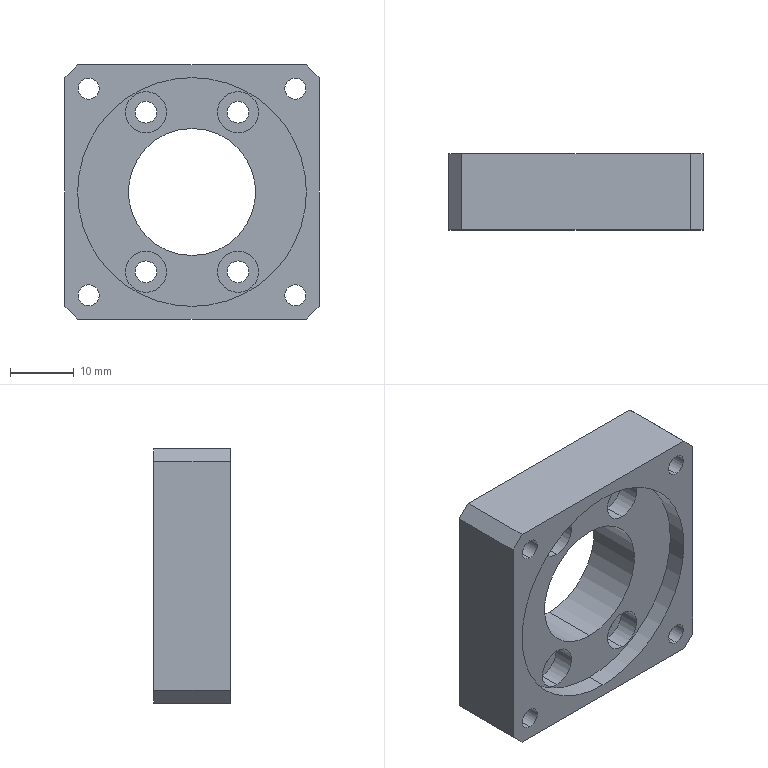Part | STEP file | 06-11 motor flange | 1 solid | 43 faces | box 40 x 12 x 40 mm | volume 12158 mm3 | cylinder 28 | plane 15 | commonest cylinder face diameters 3.3 x8 3.4 x8 6.5 x8 20 x2 36 x2
STEP:
#1=CARTESIAN_POINT('',(-16.263,12.,17.913));
#2=VERTEX_POINT('',#1);
#3=CARTESIAN_POINT('',(-16.263,12.,14.613));
#4=VERTEX_POINT('',#3);
#5=CARTESIAN_POINT('',(-16.263,12.,16.263));
#6=DIRECTION('',(0.,-1.,0.));
#7=DIRECTION('',(0.,0.,-1.));
#8=AXIS2_PLACEMENT_3D('',#5,#6,#7);
#9=CIRCLE('',#8,1.65);
#10=EDGE_CURVE('',#2,#4,#9,.T.);
#11=ORIENTED_EDGE('',*,*,#10,.F.);
#12=CARTESIAN_POINT('',(-16.263,0.,17.913));
#13=VERTEX_POINT('',#12);
#14=CARTESIAN_POINT('',(-16.263,0.,17.913));
#15=DIRECTION('',(0.,-1.,0.));
#16=VECTOR('',#15,1000.);
#17=LINE('',#14,#16);
#18=EDGE_CURVE('',#2,#13,#17,.T.);
#19=ORIENTED_EDGE('',*,*,#18,.T.);
#20=CARTESIAN_POINT('',(-16.263,0.,14.613));
#21=VERTEX_POINT('',#20);
#22=CARTESIAN_POINT('',(-16.263,0.,16.263));
#23=DIRECTION('',(0.,-1.,0.));
#24=DIRECTION('',(0.,0.,-1.));
#25=AXIS2_PLACEMENT_3D('',#22,#23,#24);
#26=CIRCLE('',#25,1.65);
#27=EDGE_CURVE('',#13,#21,#26,.T.);
#28=ORIENTED_EDGE('',*,*,#27,.T.);
#29=CARTESIAN_POINT('',(-16.263,0.,14.613));
#30=DIRECTION('',(0.,-1.,0.));
#31=VECTOR('',#30,1000.);
#32=LINE('',#29,#31);
#33=EDGE_CURVE('',#4,#21,#32,.T.);
#34=ORIENTED_EDGE('',*,*,#33,.F.);
#35=EDGE_LOOP('',(#11,#19,#28,#34));
#36=FACE_OUTER_BOUND('',#35,.T.);
#37=CARTESIAN_POINT('',(-16.263,0.,16.263));
#38=DIRECTION('',(0.,-1.,0.));
#39=DIRECTION('',(0.,0.,-1.));
#40=AXIS2_PLACEMENT_3D('',#37,#38,#39);
#41=CYLINDRICAL_SURFACE('',#40,1.65);
#42=ADVANCED_FACE('',(#36),#41,.F.);
#43=CARTESIAN_POINT('',(-16.263,12.,-14.613));
#44=VERTEX_POINT('',#43);
#45=CARTESIAN_POINT('',(-16.263,12.,-17.913));
#46=VERTEX_POINT('',#45);
#47=CARTESIAN_POINT('',(-16.263,12.,-16.263));
#48=DIRECTION('',(0.,-1.,0.));
#49=DIRECTION('',(0.,0.,-1.));
#50=AXIS2_PLACEMENT_3D('',#47,#48,#49);
#51=CIRCLE('',#50,1.65);
#52=EDGE_CURVE('',#44,#46,#51,.T.);
#53=ORIENTED_EDGE('',*,*,#52,.F.);
#54=CARTESIAN_POINT('',(-16.263,0.,-14.613));
#55=VERTEX_POINT('',#54);
#56=CARTESIAN_POINT('',(-16.263,0.,-14.613));
#57=DIRECTION('',(0.,-1.,0.));
#58=VECTOR('',#57,1000.);
#59=LINE('',#56,#58);
#60=EDGE_CURVE('',#44,#55,#59,.T.);
#61=ORIENTED_EDGE('',*,*,#60,.T.);
#62=CARTESIAN_POINT('',(-16.263,0.,-17.913));
#63=VERTEX_POINT('',#62);
#64=CARTESIAN_POINT('',(-16.263,0.,-16.263));
#65=DIRECTION('',(0.,-1.,0.));
#66=DIRECTION('',(0.,0.,-1.));
#67=AXIS2_PLACEMENT_3D('',#64,#65,#66);
#68=CIRCLE('',#67,1.65);
#69=EDGE_CURVE('',#55,#63,#68,.T.);
#70=ORIENTED_EDGE('',*,*,#69,.T.);
#71=CARTESIAN_POINT('',(-16.263,0.,-17.913));
#72=DIRECTION('',(0.,-1.,0.));
#73=VECTOR('',#72,1000.);
#74=LINE('',#71,#73);
#75=EDGE_CURVE('',#46,#63,#74,.T.);
#76=ORIENTED_EDGE('',*,*,#75,.F.);
#77=EDGE_LOOP('',(#53,#61,#70,#76));
#78=FACE_OUTER_BOUND('',#77,.T.);
#79=CARTESIAN_POINT('',(-16.263,0.,-16.263));
#80=DIRECTION('',(0.,-1.,0.));
#81=DIRECTION('',(0.,0.,-1.));
#82=AXIS2_PLACEMENT_3D('',#79,#80,#81);
#83=CYLINDRICAL_SURFACE('',#82,1.65);
#84=ADVANCED_FACE('',(#78),#83,.F.);
#85=CARTESIAN_POINT('',(16.263,12.,-14.613));
#86=VERTEX_POINT('',#85);
#87=CARTESIAN_POINT('',(16.263,12.,-17.913));
#88=VERTEX_POINT('',#87);
#89=CARTESIAN_POINT('',(16.263,12.,-16.263));
#90=DIRECTION('',(0.,-1.,0.));
#91=DIRECTION('',(0.,0.,-1.));
#92=AXIS2_PLACEMENT_3D('',#89,#90,#91);
#93=CIRCLE('',#92,1.65);
#94=EDGE_CURVE('',#86,#88,#93,.T.);
#95=ORIENTED_EDGE('',*,*,#94,.F.);
#96=CARTESIAN_POINT('',(16.263,0.,-14.613));
#97=VERTEX_POINT('',#96);
#98=CARTESIAN_POINT('',(16.263,0.,-14.613));
#99=DIRECTION('',(0.,-1.,0.));
#100=VECTOR('',#99,1000.);
#101=LINE('',#98,#100);
#102=EDGE_CURVE('',#86,#97,#101,.T.);
#103=ORIENTED_EDGE('',*,*,#102,.T.);
#104=CARTESIAN_POINT('',(16.263,0.,-17.913));
#105=VERTEX_POINT('',#104);
#106=CARTESIAN_POINT('',(16.263,0.,-16.263));
#107=DIRECTION('',(0.,-1.,0.));
#108=DIRECTION('',(0.,0.,-1.));
#109=AXIS2_PLACEMENT_3D('',#106,#107,#108);
#110=CIRCLE('',#109,1.65);
#111=EDGE_CURVE('',#97,#105,#110,.T.);
#112=ORIENTED_EDGE('',*,*,#111,.T.);
#113=CARTESIAN_POINT('',(16.263,0.,-17.913));
#114=DIRECTION('',(0.,-1.,0.));
#115=VECTOR('',#114,1000.);
#116=LINE('',#113,#115);
#117=EDGE_CURVE('',#88,#105,#116,.T.);
#118=ORIENTED_EDGE('',*,*,#117,.F.);
#119=EDGE_LOOP('',(#95,#103,#112,#118));
#120=FACE_OUTER_BOUND('',#119,.T.);
#121=CARTESIAN_POINT('',(16.263,0.,-16.263));
#122=DIRECTION('',(0.,-1.,0.));
#123=DIRECTION('',(0.,0.,-1.));
#124=AXIS2_PLACEMENT_3D('',#121,#122,#123);
#125=CYLINDRICAL_SURFACE('',#124,1.65);
#126=ADVANCED_FACE('',(#120),#125,.F.);
#127=CARTESIAN_POINT('',(16.263,12.,17.913));
#128=VERTEX_POINT('',#127);
#129=CARTESIAN_POINT('',(16.263,12.,14.613));
#130=VERTEX_POINT('',#129);
#131=CARTESIAN_POINT('',(16.263,12.,16.263));
#132=DIRECTION('',(0.,-1.,0.));
#133=DIRECTION('',(0.,0.,-1.));
#134=AXIS2_PLACEMENT_3D('',#131,#132,#133);
#135=CIRCLE('',#134,1.65);
#136=EDGE_CURVE('',#128,#130,#135,.T.);
#137=ORIENTED_EDGE('',*,*,#136,.F.);
#138=CARTESIAN_POINT('',(16.263,0.,17.913));
#139=VERTEX_POINT('',#138);
#140=CARTESIAN_POINT('',(16.263,0.,17.913));
#141=DIRECTION('',(0.,-1.,0.));
#142=VECTOR('',#141,1000.);
#143=LINE('',#140,#142);
#144=EDGE_CURVE('',#128,#139,#143,.T.);
#145=ORIENTED_EDGE('',*,*,#144,.T.);
#146=CARTESIAN_POINT('',(16.263,0.,14.613));
#147=VERTEX_POINT('',#146);
#148=CARTESIAN_POINT('',(16.263,0.,16.263));
#149=DIRECTION('',(0.,-1.,0.));
#150=DIRECTION('',(0.,0.,-1.));
#151=AXIS2_PLACEMENT_3D('',#148,#149,#150);
#152=CIRCLE('',#151,1.65);
#153=EDGE_CURVE('',#139,#147,#152,.T.);
#154=ORIENTED_EDGE('',*,*,#153,.T.);
#155=CARTESIAN_POINT('',(16.263,0.,14.613));
#156=DIRECTION('',(0.,-1.,0.));
#157=VECTOR('',#156,1000.);
#158=LINE('',#155,#157);
#159=EDGE_CURVE('',#130,#147,#158,.T.);
#160=ORIENTED_EDGE('',*,*,#159,.F.);
#161=EDGE_LOOP('',(#137,#145,#154,#160));
#162=FACE_OUTER_BOUND('',#161,.T.);
#163=CARTESIAN_POINT('',(16.263,0.,16.263));
#164=DIRECTION('',(0.,-1.,0.));
#165=DIRECTION('',(0.,0.,-1.));
#166=AXIS2_PLACEMENT_3D('',#163,#164,#165);
#167=CYLINDRICAL_SURFACE('',#166,1.65);
#168=ADVANCED_FACE('',(#162),#167,.F.);
#169=CARTESIAN_POINT('',(7.25,6.4,15.807));
#170=VERTEX_POINT('',#169);
#171=CARTESIAN_POINT('',(7.25,6.4,9.307));
#172=VERTEX_POINT('',#171);
#173=CARTESIAN_POINT('',(7.25,6.4,12.557));
#174=DIRECTION('',(0.,-1.,0.));
#175=DIRECTION('',(0.,0.,-1.));
#176=AXIS2_PLACEMENT_3D('',#173,#174,#175);
#177=CIRCLE('',#176,3.25);
#178=EDGE_CURVE('',#170,#172,#177,.T.);
#179=ORIENTED_EDGE('',*,*,#178,.F.);
#180=CARTESIAN_POINT('',(7.25,3.,15.807));
#181=VERTEX_POINT('',#180);
#182=CARTESIAN_POINT('',(7.25,3.,15.807));
#183=DIRECTION('',(0.,-1.,0.));
#184=VECTOR('',#183,1000.);
#185=LINE('',#182,#184);
#186=EDGE_CURVE('',#170,#181,#185,.T.);
#187=ORIENTED_EDGE('',*,*,#186,.T.);
#188=CARTESIAN_POINT('',(7.25,3.,9.307));
#189=VERTEX_POINT('',#188);
#190=CARTESIAN_POINT('',(7.25,3.,12.557));
#191=DIRECTION('',(0.,-1.,0.));
#192=DIRECTION('',(0.,0.,-1.));
#193=AXIS2_PLACEMENT_3D('',#190,#191,#192);
#194=CIRCLE('',#193,3.25);
#195=EDGE_CURVE('',#181,#189,#194,.T.);
#196=ORIENTED_EDGE('',*,*,#195,.T.);
#197=CARTESIAN_POINT('',(7.25,3.,9.307));
#198=DIRECTION('',(0.,-1.,0.));
#199=VECTOR('',#198,1000.);
#200=LINE('',#197,#199);
#201=EDGE_CURVE('',#172,#189,#200,.T.);
#202=ORIENTED_EDGE('',*,*,#201,.F.);
#203=EDGE_LOOP('',(#179,#187,#196,#202));
#204=FACE_OUTER_BOUND('',#203,.T.);
#205=CARTESIAN_POINT('',(7.25,3.,12.557));
#206=DIRECTION('',(0.,-1.,0.));
#207=DIRECTION('',(0.,0.,-1.));
#208=AXIS2_PLACEMENT_3D('',#205,#206,#207);
#209=CYLINDRICAL_SURFACE('',#208,3.25);
#210=ADVANCED_FACE('',(#204),#209,.F.);
#211=CARTESIAN_POINT('',(7.25,12.,14.257));
#212=VERTEX_POINT('',#211);
#213=CARTESIAN_POINT('',(7.25,12.,10.857));
#214=VERTEX_POINT('',#213);
#215=CARTESIAN_POINT('',(7.25,12.,12.557));
#216=DIRECTION('',(0.,-1.,0.));
#217=DIRECTION('',(0.,0.,-1.));
#218=AXIS2_PLACEMENT_3D('',#215,#216,#217);
#219=CIRCLE('',#218,1.7);
#220=EDGE_CURVE('',#212,#214,#219,.T.);
#221=ORIENTED_EDGE('',*,*,#220,.F.);
#222=CARTESIAN_POINT('',(7.25,6.4,14.257));
#223=VERTEX_POINT('',#222);
#224=CARTESIAN_POINT('',(7.25,3.,14.257));
#225=DIRECTION('',(0.,-1.,0.));
#226=VECTOR('',#225,1000.);
#227=LINE('',#224,#226);
#228=EDGE_CURVE('',#212,#223,#227,.T.);
#229=ORIENTED_EDGE('',*,*,#228,.T.);
#230=CARTESIAN_POINT('',(7.25,6.4,10.857));
#231=VERTEX_POINT('',#230);
#232=CARTESIAN_POINT('',(7.25,6.4,12.557));
#233=DIRECTION('',(0.,-1.,0.));
#234=DIRECTION('',(0.,0.,-1.));
#235=AXIS2_PLACEMENT_3D('',#232,#233,#234);
#236=CIRCLE('',#235,1.7);
#237=EDGE_CURVE('',#223,#231,#236,.T.);
#238=ORIENTED_EDGE('',*,*,#237,.T.);
#239=CARTESIAN_POINT('',(7.25,3.,10.857));
#240=DIRECTION('',(0.,-1.,0.));
#241=VECTOR('',#240,1000.);
#242=LINE('',#239,#241);
#243=EDGE_CURVE('',#214,#231,#242,.T.);
#244=ORIENTED_EDGE('',*,*,#243,.F.);
#245=EDGE_LOOP('',(#221,#229,#238,#244));
#246=FACE_OUTER_BOUND('',#245,.T.);
#247=CARTESIAN_POINT('',(7.25,3.,12.557));
#248=DIRECTION('',(0.,-1.,0.));
#249=DIRECTION('',(0.,0.,-1.));
#250=AXIS2_PLACEMENT_3D('',#247,#248,#249);
#251=CYLINDRICAL_SURFACE('',#250,1.7);
#252=ADVANCED_FACE('',(#246),#251,.F.);
#253=CARTESIAN_POINT('',(-7.25,6.4,15.807));
#254=VERTEX_POINT('',#253);
#255=CARTESIAN_POINT('',(-7.25,6.4,9.307));
#256=VERTEX_POINT('',#255);
#257=CARTESIAN_POINT('',(-7.25,6.4,12.557));
#258=DIRECTION('',(0.,-1.,0.));
#259=DIRECTION('',(0.,0.,-1.));
#260=AXIS2_PLACEMENT_3D('',#257,#258,#259);
#261=CIRCLE('',#260,3.25);
#262=EDGE_CURVE('',#254,#256,#261,.T.);
#263=ORIENTED_EDGE('',*,*,#262,.F.);
#264=CARTESIAN_POINT('',(-7.25,3.,15.807));
#265=VERTEX_POINT('',#264);
#266=CARTESIAN_POINT('',(-7.25,3.,15.807));
#267=DIRECTION('',(0.,-1.,0.));
#268=VECTOR('',#267,1000.);
#269=LINE('',#266,#268);
#270=EDGE_CURVE('',#254,#265,#269,.T.);
#271=ORIENTED_EDGE('',*,*,#270,.T.);
#272=CARTESIAN_POINT('',(-7.25,3.,9.307));
#273=VERTEX_POINT('',#272);
#274=CARTESIAN_POINT('',(-7.25,3.,12.557));
#275=DIRECTION('',(0.,-1.,0.));
#276=DIRECTION('',(0.,0.,-1.));
#277=AXIS2_PLACEMENT_3D('',#274,#275,#276);
#278=CIRCLE('',#277,3.25);
#279=EDGE_CURVE('',#265,#273,#278,.T.);
#280=ORIENTED_EDGE('',*,*,#279,.T.);
#281=CARTESIAN_POINT('',(-7.25,3.,9.307));
#282=DIRECTION('',(0.,-1.,0.));
#283=VECTOR('',#282,1000.);
#284=LINE('',#281,#283);
#285=EDGE_CURVE('',#256,#273,#284,.T.);
#286=ORIENTED_EDGE('',*,*,#285,.F.);
#287=EDGE_LOOP('',(#263,#271,#280,#286));
#288=FACE_OUTER_BOUND('',#287,.T.);
#289=CARTESIAN_POINT('',(-7.25,3.,12.557));
#290=DIRECTION('',(0.,-1.,0.));
#291=DIRECTION('',(0.,0.,-1.));
#292=AXIS2_PLACEMENT_3D('',#289,#290,#291);
#293=CYLINDRICAL_SURFACE('',#292,3.25);
#294=ADVANCED_FACE('',(#288),#293,.F.);
#295=CARTESIAN_POINT('',(-7.25,12.,14.257));
#296=VERTEX_POINT('',#295);
#297=CARTESIAN_POINT('',(-7.25,12.,10.857));
#298=VERTEX_POINT('',#297);
#299=CARTESIAN_POINT('',(-7.25,12.,12.557));
#300=DIRECTION('',(0.,-1.,0.));
#301=DIRECTION('',(0.,0.,-1.));
#302=AXIS2_PLACEMENT_3D('',#299,#300,#301);
#303=CIRCLE('',#302,1.7);
#304=EDGE_CURVE('',#296,#298,#303,.T.);
#305=ORIENTED_EDGE('',*,*,#304,.F.);
#306=CARTESIAN_POINT('',(-7.25,6.4,14.257));
#307=VERTEX_POINT('',#306);
#308=CARTESIAN_POINT('',(-7.25,3.,14.257));
#309=DIRECTION('',(0.,-1.,0.));
#310=VECTOR('',#309,1000.);
#311=LINE('',#308,#310);
#312=EDGE_CURVE('',#296,#307,#311,.T.);
#313=ORIENTED_EDGE('',*,*,#312,.T.);
#314=CARTESIAN_POINT('',(-7.25,6.4,10.857));
#315=VERTEX_POINT('',#314);
#316=CARTESIAN_POINT('',(-7.25,6.4,12.557));
#317=DIRECTION('',(0.,-1.,0.));
#318=DIRECTION('',(0.,0.,-1.));
#319=AXIS2_PLACEMENT_3D('',#316,#317,#318);
#320=CIRCLE('',#319,1.7);
#321=EDGE_CURVE('',#307,#315,#320,.T.);
#322=ORIENTED_EDGE('',*,*,#321,.T.);
#323=CARTESIAN_POINT('',(-7.25,3.,10.857));
#324=DIRECTION('',(0.,-1.,0.));
#325=VECTOR('',#324,1000.);
#326=LINE('',#323,#325);
#327=EDGE_CURVE('',#298,#315,#326,.T.);
#328=ORIENTED_EDGE('',*,*,#327,.F.);
#329=EDGE_LOOP('',(#305,#313,#322,#328));
#330=FACE_OUTER_BOUND('',#329,.T.);
#331=CARTESIAN_POINT('',(-7.25,3.,12.557));
#332=DIRECTION('',(0.,-1.,0.));
#333=DIRECTION('',(0.,0.,-1.));
#334=AXIS2_PLACEMENT_3D('',#331,#332,#333);
#335=CYLINDRICAL_SURFACE('',#334,1.7);
#336=ADVANCED_FACE('',(#330),#335,.F.);
#337=CARTESIAN_POINT('',(-7.25,6.4,-9.307));
#338=VERTEX_POINT('',#337);
#339=CARTESIAN_POINT('',(-7.25,6.4,-15.807));
#340=VERTEX_POINT('',#339);
#341=CARTESIAN_POINT('',(-7.25,6.4,-12.557));
#342=DIRECTION('',(0.,-1.,0.));
#343=DIRECTION('',(0.,0.,-1.));
#344=AXIS2_PLACEMENT_3D('',#341,#342,#343);
#345=CIRCLE('',#344,3.25);
#346=EDGE_CURVE('',#338,#340,#345,.T.);
#347=ORIENTED_EDGE('',*,*,#346,.F.);
#348=CARTESIAN_POINT('',(-7.25,3.,-9.307));
#349=VERTEX_POINT('',#348);
#350=CARTESIAN_POINT('',(-7.25,3.,-9.307));
#351=DIRECTION('',(0.,-1.,0.));
#352=VECTOR('',#351,1000.);
#353=LINE('',#350,#352);
#354=EDGE_CURVE('',#338,#349,#353,.T.);
#355=ORIENTED_EDGE('',*,*,#354,.T.);
#356=CARTESIAN_POINT('',(-7.25,3.,-15.807));
#357=VERTEX_POINT('',#356);
#358=CARTESIAN_POINT('',(-7.25,3.,-12.557));
#359=DIRECTION('',(0.,-1.,0.));
#360=DIRECTION('',(0.,0.,-1.));
#361=AXIS2_PLACEMENT_3D('',#358,#359,#360);
#362=CIRCLE('',#361,3.25);
#363=EDGE_CURVE('',#349,#357,#362,.T.);
#364=ORIENTED_EDGE('',*,*,#363,.T.);
#365=CARTESIAN_POINT('',(-7.25,3.,-15.807));
#366=DIRECTION('',(0.,-1.,0.));
#367=VECTOR('',#366,1000.);
#368=LINE('',#365,#367);
#369=EDGE_CURVE('',#340,#357,#368,.T.);
#370=ORIENTED_EDGE('',*,*,#369,.F.);
#371=EDGE_LOOP('',(#347,#355,#364,#370));
#372=FACE_OUTER_BOUND('',#371,.T.);
#373=CARTESIAN_POINT('',(-7.25,3.,-12.557));
#374=DIRECTION('',(0.,-1.,0.));
#375=DIRECTION('',(0.,0.,-1.));
#376=AXIS2_PLACEMENT_3D('',#373,#374,#375);
#377=CYLINDRICAL_SURFACE('',#376,3.25);
#378=ADVANCED_FACE('',(#372),#377,.F.);
#379=CARTESIAN_POINT('',(-7.25,12.,-10.857));
#380=VERTEX_POINT('',#379);
#381=CARTESIAN_POINT('',(-7.25,12.,-14.257));
#382=VERTEX_POINT('',#381);
#383=CARTESIAN_POINT('',(-7.25,12.,-12.557));
#384=DIRECTION('',(0.,-1.,0.));
#385=DIRECTION('',(0.,0.,-1.));
#386=AXIS2_PLACEMENT_3D('',#383,#384,#385);
#387=CIRCLE('',#386,1.7);
#388=EDGE_CURVE('',#380,#382,#387,.T.);
#389=ORIENTED_EDGE('',*,*,#388,.F.);
#390=CARTESIAN_POINT('',(-7.25,6.4,-10.857));
#391=VERTEX_POINT('',#390);
#392=CARTESIAN_POINT('',(-7.25,3.,-10.857));
#393=DIRECTION('',(0.,-1.,0.));
#394=VECTOR('',#393,1000.);
#395=LINE('',#392,#394);
#396=EDGE_CURVE('',#380,#391,#395,.T.);
#397=ORIENTED_EDGE('',*,*,#396,.T.);
#398=CARTESIAN_POINT('',(-7.25,6.4,-14.257));
#399=VERTEX_POINT('',#398);
#400=CARTESIAN_POINT('',(-7.25,6.4,-12.557));
#401=DIRECTION('',(0.,-1.,0.));
#402=DIRECTION('',(0.,0.,-1.));
#403=AXIS2_PLACEMENT_3D('',#400,#401,#402);
#404=CIRCLE('',#403,1.7);
#405=EDGE_CURVE('',#391,#399,#404,.T.);
#406=ORIENTED_EDGE('',*,*,#405,.T.);
#407=CARTESIAN_POINT('',(-7.25,3.,-14.257));
#408=DIRECTION('',(0.,-1.,0.));
#409=VECTOR('',#408,1000.);
#410=LINE('',#407,#409);
#411=EDGE_CURVE('',#382,#399,#410,.T.);
#412=ORIENTED_EDGE('',*,*,#411,.F.);
#413=EDGE_LOOP('',(#389,#397,#406,#412));
#414=FACE_OUTER_BOUND('',#413,.T.);
#415=CARTESIAN_POINT('',(-7.25,3.,-12.557));
#416=DIRECTION('',(0.,-1.,0.));
#417=DIRECTION('',(0.,0.,-1.));
#418=AXIS2_PLACEMENT_3D('',#415,#416,#417);
#419=CYLINDRICAL_SURFACE('',#418,1.7);
#420=ADVANCED_FACE('',(#414),#419,.F.);
#421=CARTESIAN_POINT('',(7.25,6.4,-9.307));
#422=VERTEX_POINT('',#421);
#423=CARTESIAN_POINT('',(7.25,6.4,-15.807));
#424=VERTEX_POINT('',#423);
#425=CARTESIAN_POINT('',(7.25,6.4,-12.557));
#426=DIRECTION('',(0.,-1.,0.));
#427=DIRECTION('',(0.,0.,-1.));
#428=AXIS2_PLACEMENT_3D('',#425,#426,#427);
#429=CIRCLE('',#428,3.25);
#430=EDGE_CURVE('',#422,#424,#429,.T.);
#431=ORIENTED_EDGE('',*,*,#430,.F.);
#432=CARTESIAN_POINT('',(7.25,3.,-9.307));
#433=VERTEX_POINT('',#432);
#434=CARTESIAN_POINT('',(7.25,3.,-9.307));
#435=DIRECTION('',(0.,-1.,0.));
#436=VECTOR('',#435,1000.);
#437=LINE('',#434,#436);
#438=EDGE_CURVE('',#422,#433,#437,.T.);
#439=ORIENTED_EDGE('',*,*,#438,.T.);
#440=CARTESIAN_POINT('',(7.25,3.,-15.807));
#441=VERTEX_POINT('',#440);
#442=CARTESIAN_POINT('',(7.25,3.,-12.557));
#443=DIRECTION('',(0.,-1.,0.));
#444=DIRECTION('',(0.,0.,-1.));
#445=AXIS2_PLACEMENT_3D('',#442,#443,#444);
#446=CIRCLE('',#445,3.25);
#447=EDGE_CURVE('',#433,#441,#446,.T.);
#448=ORIENTED_EDGE('',*,*,#447,.T.);
#449=CARTESIAN_POINT('',(7.25,3.,-15.807));
#450=DIRECTION('',(0.,-1.,0.));
#451=VECTOR('',#450,1000.);
#452=LINE('',#449,#451);
#453=EDGE_CURVE('',#424,#441,#452,.T.);
#454=ORIENTED_EDGE('',*,*,#453,.F.);
#455=EDGE_LOOP('',(#431,#439,#448,#454));
#456=FACE_OUTER_BOUND('',#455,.T.);
#457=CARTESIAN_POINT('',(7.25,3.,-12.557));
#458=DIRECTION('',(0.,-1.,0.));
#459=DIRECTION('',(0.,0.,-1.));
#460=AXIS2_PLACEMENT_3D('',#457,#458,#459);
#461=CYLINDRICAL_SURFACE('',#460,3.25);
#462=ADVANCED_FACE('',(#456),#461,.F.);
#463=CARTESIAN_POINT('',(7.25,12.,-10.857));
#464=VERTEX_POINT('',#463);
#465=CARTESIAN_POINT('',(7.25,12.,-14.257));
#466=VERTEX_POINT('',#465);
#467=CARTESIAN_POINT('',(7.25,12.,-12.557));
#468=DIRECTION('',(0.,-1.,0.));
#469=DIRECTION('',(0.,0.,-1.));
#470=AXIS2_PLACEMENT_3D('',#467,#468,#469);
#471=CIRCLE('',#470,1.7);
#472=EDGE_CURVE('',#464,#466,#471,.T.);
#473=ORIENTED_EDGE('',*,*,#472,.F.);
#474=CARTESIAN_POINT('',(7.25,6.4,-10.857));
#475=VERTEX_POINT('',#474);
#476=CARTESIAN_POINT('',(7.25,3.,-10.857));
#477=DIRECTION('',(0.,-1.,0.));
#478=VECTOR('',#477,1000.);
#479=LINE('',#476,#478);
#480=EDGE_CURVE('',#464,#475,#479,.T.);
#481=ORIENTED_EDGE('',*,*,#480,.T.);
#482=CARTESIAN_POINT('',(7.25,6.4,-14.257));
#483=VERTEX_POINT('',#482);
#484=CARTESIAN_POINT('',(7.25,6.4,-12.557));
#485=DIRECTION('',(0.,-1.,0.));
#486=DIRECTION('',(0.,0.,-1.));
#487=AXIS2_PLACEMENT_3D('',#484,#485,#486);
#488=CIRCLE('',#487,1.7);
#489=EDGE_CURVE('',#475,#483,#488,.T.);
#490=ORIENTED_EDGE('',*,*,#489,.T.);
#491=CARTESIAN_POINT('',(7.25,3.,-14.257));
#492=DIRECTION('',(0.,-1.,0.));
#493=VECTOR('',#492,1000.);
#494=LINE('',#491,#493);
#495=EDGE_CURVE('',#466,#483,#494,.T.);
#496=ORIENTED_EDGE('',*,*,#495,.F.);
#497=EDGE_LOOP('',(#473,#481,#490,#496));
#498=FACE_OUTER_BOUND('',#497,.T.);
#499=CARTESIAN_POINT('',(7.25,3.,-12.557));
#500=DIRECTION('',(0.,-1.,0.));
#501=DIRECTION('',(0.,0.,-1.));
#502=AXIS2_PLACEMENT_3D('',#499,#500,#501);
#503=CYLINDRICAL_SURFACE('',#502,1.7);
#504=ADVANCED_FACE('',(#498),#503,.F.);
#505=CARTESIAN_POINT('',(0.,3.,18.));
#506=VERTEX_POINT('',#505);
#507=CARTESIAN_POINT('',(0.,3.,-18.));
#508=VERTEX_POINT('',#507);
#509=CARTESIAN_POINT('',(0.,3.,0.));
#510=DIRECTION('',(0.,-1.,0.));
#511=DIRECTION('',(0.,0.,-1.));
#512=AXIS2_PLACEMENT_3D('',#509,#510,#511);
#513=CIRCLE('',#512,18.);
#514=EDGE_CURVE('',#506,#508,#513,.T.);
#515=ORIENTED_EDGE('',*,*,#514,.F.);
#516=CARTESIAN_POINT('',(0.,0.,18.));
#517=VERTEX_POINT('',#516);
#518=CARTESIAN_POINT('',(0.,3.,18.));
#519=DIRECTION('',(0.,-1.,0.));
#520=VECTOR('',#519,1000.);
#521=LINE('',#518,#520);
#522=EDGE_CURVE('',#506,#517,#521,.T.);
#523=ORIENTED_EDGE('',*,*,#522,.T.);
#524=CARTESIAN_POINT('',(0.,0.,-18.));
#525=VERTEX_POINT('',#524);
#526=CARTESIAN_POINT('',(0.,0.,0.));
#527=DIRECTION('',(0.,-1.,0.));
#528=DIRECTION('',(0.,0.,-1.));
#529=AXIS2_PLACEMENT_3D('',#526,#527,#528);
#530=CIRCLE('',#529,18.);
#531=EDGE_CURVE('',#517,#525,#530,.T.);
#532=ORIENTED_EDGE('',*,*,#531,.T.);
#533=CARTESIAN_POINT('',(0.,3.,-18.));
#534=DIRECTION('',(0.,-1.,0.));
#535=VECTOR('',#534,1000.);
#536=LINE('',#533,#535);
#537=EDGE_CURVE('',#508,#525,#536,.T.);
#538=ORIENTED_EDGE('',*,*,#537,.F.);
#539=EDGE_LOOP('',(#515,#523,#532,#538));
#540=FACE_OUTER_BOUND('',#539,.T.);
#541=CARTESIAN_POINT('',(0.,3.,0.));
#542=DIRECTION('',(0.,-1.,0.));
#543=DIRECTION('',(0.,0.,-1.));
#544=AXIS2_PLACEMENT_3D('',#541,#542,#543);
#545=CYLINDRICAL_SURFACE('',#544,18.);
#546=ADVANCED_FACE('',(#540),#545,.F.);
#547=CARTESIAN_POINT('',(0.,12.,-10.));
#548=VERTEX_POINT('',#547);
#549=CARTESIAN_POINT('',(0.,12.,10.));
#550=VERTEX_POINT('',#549);
#551=CARTESIAN_POINT('',(0.,12.,0.));
#552=DIRECTION('',(0.,1.,0.));
#553=DIRECTION('',(0.,0.,1.));
#554=AXIS2_PLACEMENT_3D('',#551,#552,#553);
#555=CIRCLE('',#554,10.);
#556=EDGE_CURVE('',#548,#550,#555,.T.);
#557=ORIENTED_EDGE('',*,*,#556,.T.);
#558=CARTESIAN_POINT('',(0.,3.,10.));
#559=VERTEX_POINT('',#558);
#560=CARTESIAN_POINT('',(0.,12.,10.));
#561=DIRECTION('',(0.,-1.,0.));
#562=VECTOR('',#561,1000.);
#563=LINE('',#560,#562);
#564=EDGE_CURVE('',#550,#559,#563,.T.);
#565=ORIENTED_EDGE('',*,*,#564,.T.);
#566=CARTESIAN_POINT('',(0.,3.,-10.));
#567=VERTEX_POINT('',#566);
#568=CARTESIAN_POINT('',(0.,3.,0.));
#569=DIRECTION('',(0.,-1.,0.));
#570=DIRECTION('',(0.,0.,-1.));
#571=AXIS2_PLACEMENT_3D('',#568,#569,#570);
#572=CIRCLE('',#571,10.);
#573=EDGE_CURVE('',#559,#567,#572,.T.);
#574=ORIENTED_EDGE('',*,*,#573,.T.);
#575=CARTESIAN_POINT('',(0.,12.,-10.));
#576=DIRECTION('',(0.,-1.,0.));
#577=VECTOR('',#576,1000.);
#578=LINE('',#575,#577);
#579=EDGE_CURVE('',#548,#567,#578,.T.);
#580=ORIENTED_EDGE('',*,*,#579,.F.);
#581=EDGE_LOOP('',(#557,#565,#574,#580));
#582=FACE_OUTER_BOUND('',#581,.T.);
#583=CARTESIAN_POINT('',(0.,12.,0.));
#584=DIRECTION('',(0.,-1.,0.));
#585=DIRECTION('',(0.,0.,-1.));
#586=AXIS2_PLACEMENT_3D('',#583,#584,#585);
#587=CYLINDRICAL_SURFACE('',#586,10.);
#588=ADVANCED_FACE('',(#582),#587,.F.);
#589=ORIENTED_EDGE('',*,*,#564,.F.);
#590=CARTESIAN_POINT('',(0.,12.,0.));
#591=DIRECTION('',(0.,1.,0.));
#592=DIRECTION('',(0.,0.,1.));
#593=AXIS2_PLACEMENT_3D('',#590,#591,#592);
#594=CIRCLE('',#593,10.);
#595=EDGE_CURVE('',#550,#548,#594,.T.);
#596=ORIENTED_EDGE('',*,*,#595,.T.);
#597=ORIENTED_EDGE('',*,*,#579,.T.);
#598=CARTESIAN_POINT('',(0.,3.,0.));
#599=DIRECTION('',(0.,-1.,0.));
#600=DIRECTION('',(0.,0.,-1.));
#601=AXIS2_PLACEMENT_3D('',#598,#599,#600);
#602=CIRCLE('',#601,10.);
#603=EDGE_CURVE('',#567,#559,#602,.T.);
#604=ORIENTED_EDGE('',*,*,#603,.T.);
#605=EDGE_LOOP('',(#589,#596,#597,#604));
#606=FACE_OUTER_BOUND('',#605,.T.);
#607=CARTESIAN_POINT('',(0.,12.,0.));
#608=DIRECTION('',(0.,-1.,0.));
#609=DIRECTION('',(0.,0.,-1.));
#610=AXIS2_PLACEMENT_3D('',#607,#608,#609);
#611=CYLINDRICAL_SURFACE('',#610,10.);
#612=ADVANCED_FACE('',(#606),#611,.F.);
#613=CARTESIAN_POINT('',(-16.263,12.,16.263));
#614=DIRECTION('',(0.,-1.,0.));
#615=DIRECTION('',(0.,0.,-1.));
#616=AXIS2_PLACEMENT_3D('',#613,#614,#615);
#617=CIRCLE('',#616,1.65);
#618=EDGE_CURVE('',#4,#2,#617,.T.);
#619=ORIENTED_EDGE('',*,*,#618,.T.);
#620=ORIENTED_EDGE('',*,*,#10,.T.);
#621=EDGE_LOOP('',(#619,#620));
#622=FACE_BOUND('',#621,.T.);
#623=CARTESIAN_POINT('',(-16.263,12.,-16.263));
#624=DIRECTION('',(0.,-1.,0.));
#625=DIRECTION('',(0.,0.,-1.));
#626=AXIS2_PLACEMENT_3D('',#623,#624,#625);
#627=CIRCLE('',#626,1.65);
#628=EDGE_CURVE('',#46,#44,#627,.T.);
#629=ORIENTED_EDGE('',*,*,#628,.T.);
#630=ORIENTED_EDGE('',*,*,#52,.T.);
#631=EDGE_LOOP('',(#629,#630));
#632=FACE_BOUND('',#631,.T.);
#633=CARTESIAN_POINT('',(16.263,12.,-16.263));
#634=DIRECTION('',(0.,-1.,0.));
#635=DIRECTION('',(0.,0.,-1.));
#636=AXIS2_PLACEMENT_3D('',#633,#634,#635);
#637=CIRCLE('',#636,1.65);
#638=EDGE_CURVE('',#88,#86,#637,.T.);
#639=ORIENTED_EDGE('',*,*,#638,.T.);
#640=ORIENTED_EDGE('',*,*,#94,.T.);
#641=EDGE_LOOP('',(#639,#640));
#642=FACE_BOUND('',#641,.T.);
#643=CARTESIAN_POINT('',(16.263,12.,16.263));
#644=DIRECTION('',(0.,-1.,0.));
#645=DIRECTION('',(0.,0.,-1.));
#646=AXIS2_PLACEMENT_3D('',#643,#644,#645);
#647=CIRCLE('',#646,1.65);
#648=EDGE_CURVE('',#130,#128,#647,.T.);
#649=ORIENTED_EDGE('',*,*,#648,.T.);
#650=ORIENTED_EDGE('',*,*,#136,.T.);
#651=EDGE_LOOP('',(#649,#650));
#652=FACE_BOUND('',#651,.T.);
#653=CARTESIAN_POINT('',(7.25,12.,12.557));
#654=DIRECTION('',(0.,-1.,0.));
#655=DIRECTION('',(0.,0.,-1.));
#656=AXIS2_PLACEMENT_3D('',#653,#654,#655);
#657=CIRCLE('',#656,1.7);
#658=EDGE_CURVE('',#214,#212,#657,.T.);
#659=ORIENTED_EDGE('',*,*,#658,.T.);
#660=ORIENTED_EDGE('',*,*,#220,.T.);
#661=EDGE_LOOP('',(#659,#660));
#662=FACE_BOUND('',#661,.T.);
#663=CARTESIAN_POINT('',(-7.25,12.,12.557));
#664=DIRECTION('',(0.,-1.,0.));
#665=DIRECTION('',(0.,0.,-1.));
#666=AXIS2_PLACEMENT_3D('',#663,#664,#665);
#667=CIRCLE('',#666,1.7);
#668=EDGE_CURVE('',#298,#296,#667,.T.);
#669=ORIENTED_EDGE('',*,*,#668,.T.);
#670=ORIENTED_EDGE('',*,*,#304,.T.);
#671=EDGE_LOOP('',(#669,#670));
#672=FACE_BOUND('',#671,.T.);
#673=CARTESIAN_POINT('',(-7.25,12.,-12.557));
#674=DIRECTION('',(0.,-1.,0.));
#675=DIRECTION('',(0.,0.,-1.));
#676=AXIS2_PLACEMENT_3D('',#673,#674,#675);
#677=CIRCLE('',#676,1.7);
#678=EDGE_CURVE('',#382,#380,#677,.T.);
#679=ORIENTED_EDGE('',*,*,#678,.T.);
#680=ORIENTED_EDGE('',*,*,#388,.T.);
#681=EDGE_LOOP('',(#679,#680));
#682=FACE_BOUND('',#681,.T.);
#683=CARTESIAN_POINT('',(7.25,12.,-12.557));
#684=DIRECTION('',(0.,-1.,0.));
#685=DIRECTION('',(0.,0.,-1.));
#686=AXIS2_PLACEMENT_3D('',#683,#684,#685);
#687=CIRCLE('',#686,1.7);
#688=EDGE_CURVE('',#466,#464,#687,.T.);
#689=ORIENTED_EDGE('',*,*,#688,.T.);
#690=ORIENTED_EDGE('',*,*,#472,.T.);
#691=EDGE_LOOP('',(#689,#690));
#692=FACE_BOUND('',#691,.T.);
#693=CARTESIAN_POINT('',(-20.,12.,-18.));
#694=VERTEX_POINT('',#693);
#695=CARTESIAN_POINT('',(-20.,12.,18.));
#696=VERTEX_POINT('',#695);
#697=CARTESIAN_POINT('',(-20.,12.,-20.));
#698=DIRECTION('',(0.,0.,1.));
#699=VECTOR('',#698,1000.);
#700=LINE('',#697,#699);
#701=EDGE_CURVE('',#694,#696,#700,.T.);
#702=ORIENTED_EDGE('',*,*,#701,.T.);
#703=CARTESIAN_POINT('',(-18.,12.,20.));
#704=VERTEX_POINT('',#703);
#705=CARTESIAN_POINT('',(1.,12.,39.));
#706=DIRECTION('',(0.7071,0.,0.7071));
#707=VECTOR('',#706,1000.);
#708=LINE('',#705,#707);
#709=EDGE_CURVE('',#696,#704,#708,.T.);
#710=ORIENTED_EDGE('',*,*,#709,.T.);
#711=CARTESIAN_POINT('',(18.,12.,20.));
#712=VERTEX_POINT('',#711);
#713=CARTESIAN_POINT('',(-20.,12.,20.));
#714=DIRECTION('',(1.,0.,0.));
#715=VECTOR('',#714,1000.);
#716=LINE('',#713,#715);
#717=EDGE_CURVE('',#704,#712,#716,.T.);
#718=ORIENTED_EDGE('',*,*,#717,.T.);
#719=CARTESIAN_POINT('',(20.,12.,18.));
#720=VERTEX_POINT('',#719);
#721=CARTESIAN_POINT('',(19.,12.,19.));
#722=DIRECTION('',(0.7071,0.,-0.7071));
#723=VECTOR('',#722,1000.);
#724=LINE('',#721,#723);
#725=EDGE_CURVE('',#712,#720,#724,.T.);
#726=ORIENTED_EDGE('',*,*,#725,.T.);
#727=CARTESIAN_POINT('',(20.,12.,-18.));
#728=VERTEX_POINT('',#727);
#729=CARTESIAN_POINT('',(20.,12.,-20.));
#730=DIRECTION('',(0.,0.,-1.));
#731=VECTOR('',#730,1000.);
#732=LINE('',#729,#731);
#733=EDGE_CURVE('',#720,#728,#732,.T.);
#734=ORIENTED_EDGE('',*,*,#733,.T.);
#735=CARTESIAN_POINT('',(18.,12.,-20.));
#736=VERTEX_POINT('',#735);
#737=CARTESIAN_POINT('',(39.,12.,1.));
#738=DIRECTION('',(-0.7071,0.,-0.7071));
#739=VECTOR('',#738,1000.);
#740=LINE('',#737,#739);
#741=EDGE_CURVE('',#728,#736,#740,.T.);
#742=ORIENTED_EDGE('',*,*,#741,.T.);
#743=CARTESIAN_POINT('',(-18.,12.,-20.));
#744=VERTEX_POINT('',#743);
#745=CARTESIAN_POINT('',(-20.,12.,-20.));
#746=DIRECTION('',(-1.,0.,0.));
#747=VECTOR('',#746,1000.);
#748=LINE('',#745,#747);
#749=EDGE_CURVE('',#736,#744,#748,.T.);
#750=ORIENTED_EDGE('',*,*,#749,.T.);
#751=CARTESIAN_POINT('',(-19.,12.,-19.));
#752=DIRECTION('',(-0.7071,0.,0.7071));
#753=VECTOR('',#752,1000.);
#754=LINE('',#751,#753);
#755=EDGE_CURVE('',#744,#694,#754,.T.);
#756=ORIENTED_EDGE('',*,*,#755,.T.);
#757=EDGE_LOOP('',(#702,#710,#718,#726,#734,#742,#750,#756));
#758=FACE_OUTER_BOUND('',#757,.T.);
#759=ORIENTED_EDGE('',*,*,#556,.F.);
#760=ORIENTED_EDGE('',*,*,#595,.F.);
#761=EDGE_LOOP('',(#759,#760));
#762=FACE_BOUND('',#761,.T.);
#763=CARTESIAN_POINT('',(20.,12.,20.));
#764=DIRECTION('',(0.,1.,0.));
#765=DIRECTION('',(0.,0.,1.));
#766=AXIS2_PLACEMENT_3D('',#763,#764,#765);
#767=PLANE('',#766);
#768=ADVANCED_FACE('',(#622,#632,#642,#652,#662,#672,#682,#692,#758,#762),#767,.T.);
#769=CARTESIAN_POINT('',(-16.263,0.,16.263));
#770=DIRECTION('',(0.,-1.,0.));
#771=DIRECTION('',(0.,0.,-1.));
#772=AXIS2_PLACEMENT_3D('',#769,#770,#771);
#773=CIRCLE('',#772,1.65);
#774=EDGE_CURVE('',#21,#13,#773,.T.);
#775=ORIENTED_EDGE('',*,*,#774,.F.);
#776=ORIENTED_EDGE('',*,*,#27,.F.);
#777=EDGE_LOOP('',(#775,#776));
#778=FACE_BOUND('',#777,.T.);
#779=CARTESIAN_POINT('',(-16.263,0.,-16.263));
#780=DIRECTION('',(0.,-1.,0.));
#781=DIRECTION('',(0.,0.,-1.));
#782=AXIS2_PLACEMENT_3D('',#779,#780,#781);
#783=CIRCLE('',#782,1.65);
#784=EDGE_CURVE('',#63,#55,#783,.T.);
#785=ORIENTED_EDGE('',*,*,#784,.F.);
#786=ORIENTED_EDGE('',*,*,#69,.F.);
#787=EDGE_LOOP('',(#785,#786));
#788=FACE_BOUND('',#787,.T.);
#789=CARTESIAN_POINT('',(16.263,0.,-16.263));
#790=DIRECTION('',(0.,-1.,0.));
#791=DIRECTION('',(0.,0.,-1.));
#792=AXIS2_PLACEMENT_3D('',#789,#790,#791);
#793=CIRCLE('',#792,1.65);
#794=EDGE_CURVE('',#105,#97,#793,.T.);
#795=ORIENTED_EDGE('',*,*,#794,.F.);
#796=ORIENTED_EDGE('',*,*,#111,.F.);
#797=EDGE_LOOP('',(#795,#796));
#798=FACE_BOUND('',#797,.T.);
#799=CARTESIAN_POINT('',(16.263,0.,16.263));
#800=DIRECTION('',(0.,-1.,0.));
#801=DIRECTION('',(0.,0.,-1.));
#802=AXIS2_PLACEMENT_3D('',#799,#800,#801);
#803=CIRCLE('',#802,1.65);
#804=EDGE_CURVE('',#147,#139,#803,.T.);
#805=ORIENTED_EDGE('',*,*,#804,.F.);
#806=ORIENTED_EDGE('',*,*,#153,.F.);
#807=EDGE_LOOP('',(#805,#806));
#808=FACE_BOUND('',#807,.T.);
#809=CARTESIAN_POINT('',(0.,0.,0.));
#810=DIRECTION('',(0.,-1.,0.));
#811=DIRECTION('',(0.,0.,-1.));
#812=AXIS2_PLACEMENT_3D('',#809,#810,#811);
#813=CIRCLE('',#812,18.);
#814=EDGE_CURVE('',#525,#517,#813,.T.);
#815=ORIENTED_EDGE('',*,*,#814,.F.);
#816=ORIENTED_EDGE('',*,*,#531,.F.);
#817=EDGE_LOOP('',(#815,#816));
#818=FACE_BOUND('',#817,.T.);
#819=CARTESIAN_POINT('',(-18.,0.,20.));
#820=VERTEX_POINT('',#819);
#821=CARTESIAN_POINT('',(18.,0.,20.));
#822=VERTEX_POINT('',#821);
#823=CARTESIAN_POINT('',(-20.,0.,20.));
#824=DIRECTION('',(1.,0.,0.));
#825=VECTOR('',#824,1000.);
#826=LINE('',#823,#825);
#827=EDGE_CURVE('',#820,#822,#826,.T.);
#828=ORIENTED_EDGE('',*,*,#827,.F.);
#829=CARTESIAN_POINT('',(-20.,0.,18.));
#830=VERTEX_POINT('',#829);
#831=CARTESIAN_POINT('',(-18.,0.,20.));
#832=DIRECTION('',(-0.7071,0.,-0.7071));
#833=VECTOR('',#832,1000.);
#834=LINE('',#831,#833);
#835=EDGE_CURVE('',#820,#830,#834,.T.);
#836=ORIENTED_EDGE('',*,*,#835,.T.);
#837=CARTESIAN_POINT('',(-20.,0.,-18.));
#838=VERTEX_POINT('',#837);
#839=CARTESIAN_POINT('',(-20.,0.,-20.));
#840=DIRECTION('',(0.,0.,1.));
#841=VECTOR('',#840,1000.);
#842=LINE('',#839,#841);
#843=EDGE_CURVE('',#838,#830,#842,.T.);
#844=ORIENTED_EDGE('',*,*,#843,.F.);
#845=CARTESIAN_POINT('',(-18.,0.,-20.));
#846=VERTEX_POINT('',#845);
#847=CARTESIAN_POINT('',(-20.,0.,-18.));
#848=DIRECTION('',(0.7071,0.,-0.7071));
#849=VECTOR('',#848,1000.);
#850=LINE('',#847,#849);
#851=EDGE_CURVE('',#838,#846,#850,.T.);
#852=ORIENTED_EDGE('',*,*,#851,.T.);
#853=CARTESIAN_POINT('',(18.,0.,-20.));
#854=VERTEX_POINT('',#853);
#855=CARTESIAN_POINT('',(-20.,0.,-20.));
#856=DIRECTION('',(-1.,0.,0.));
#857=VECTOR('',#856,1000.);
#858=LINE('',#855,#857);
#859=EDGE_CURVE('',#854,#846,#858,.T.);
#860=ORIENTED_EDGE('',*,*,#859,.F.);
#861=CARTESIAN_POINT('',(20.,0.,-18.));
#862=VERTEX_POINT('',#861);
#863=CARTESIAN_POINT('',(18.,0.,-20.));
#864=DIRECTION('',(0.7071,0.,0.7071));
#865=VECTOR('',#864,1000.);
#866=LINE('',#863,#865);
#867=EDGE_CURVE('',#854,#862,#866,.T.);
#868=ORIENTED_EDGE('',*,*,#867,.T.);
#869=CARTESIAN_POINT('',(20.,0.,18.));
#870=VERTEX_POINT('',#869);
#871=CARTESIAN_POINT('',(20.,0.,-20.));
#872=DIRECTION('',(0.,0.,-1.));
#873=VECTOR('',#872,1000.);
#874=LINE('',#871,#873);
#875=EDGE_CURVE('',#870,#862,#874,.T.);
#876=ORIENTED_EDGE('',*,*,#875,.F.);
#877=CARTESIAN_POINT('',(20.,0.,18.));
#878=DIRECTION('',(-0.7071,0.,0.7071));
#879=VECTOR('',#878,1000.);
#880=LINE('',#877,#879);
#881=EDGE_CURVE('',#870,#822,#880,.T.);
#882=ORIENTED_EDGE('',*,*,#881,.T.);
#883=EDGE_LOOP('',(#828,#836,#844,#852,#860,#868,#876,#882));
#884=FACE_OUTER_BOUND('',#883,.T.);
#885=CARTESIAN_POINT('',(20.,0.,20.));
#886=DIRECTION('',(0.,1.,0.));
#887=DIRECTION('',(0.,0.,1.));
#888=AXIS2_PLACEMENT_3D('',#885,#886,#887);
#889=PLANE('',#888);
#890=ADVANCED_FACE('',(#778,#788,#798,#808,#818,#884),#889,.F.);
#891=ORIENTED_EDGE('',*,*,#875,.T.);
#892=CARTESIAN_POINT('',(20.,12.,-18.));
#893=DIRECTION('',(0.,1.,0.));
#894=VECTOR('',#893,1000.);
#895=LINE('',#892,#894);
#896=EDGE_CURVE('',#862,#728,#895,.T.);
#897=ORIENTED_EDGE('',*,*,#896,.T.);
#898=ORIENTED_EDGE('',*,*,#733,.F.);
#899=CARTESIAN_POINT('',(20.,12.,18.));
#900=DIRECTION('',(0.,-1.,0.));
#901=VECTOR('',#900,1000.);
#902=LINE('',#899,#901);
#903=EDGE_CURVE('',#720,#870,#902,.T.);
#904=ORIENTED_EDGE('',*,*,#903,.T.);
#905=EDGE_LOOP('',(#891,#897,#898,#904));
#906=FACE_OUTER_BOUND('',#905,.T.);
#907=CARTESIAN_POINT('',(20.,12.,-20.));
#908=DIRECTION('',(-1.,0.,0.));
#909=DIRECTION('',(0.,0.,1.));
#910=AXIS2_PLACEMENT_3D('',#907,#908,#909);
#911=PLANE('',#910);
#912=ADVANCED_FACE('',(#906),#911,.F.);
#913=ORIENTED_EDGE('',*,*,#859,.T.);
#914=CARTESIAN_POINT('',(-18.,12.,-20.));
#915=DIRECTION('',(0.,1.,0.));
#916=VECTOR('',#915,1000.);
#917=LINE('',#914,#916);
#918=EDGE_CURVE('',#846,#744,#917,.T.);
#919=ORIENTED_EDGE('',*,*,#918,.T.);
#920=ORIENTED_EDGE('',*,*,#749,.F.);
#921=CARTESIAN_POINT('',(18.,12.,-20.));
#922=DIRECTION('',(0.,-1.,0.));
#923=VECTOR('',#922,1000.);
#924=LINE('',#921,#923);
#925=EDGE_CURVE('',#736,#854,#924,.T.);
#926=ORIENTED_EDGE('',*,*,#925,.T.);
#927=EDGE_LOOP('',(#913,#919,#920,#926));
#928=FACE_OUTER_BOUND('',#927,.T.);
#929=CARTESIAN_POINT('',(-20.,12.,-20.));
#930=DIRECTION('',(0.,0.,1.));
#931=DIRECTION('',(1.,0.,0.));
#932=AXIS2_PLACEMENT_3D('',#929,#930,#931);
#933=PLANE('',#932);
#934=ADVANCED_FACE('',(#928),#933,.F.);
#935=ORIENTED_EDGE('',*,*,#843,.T.);
#936=CARTESIAN_POINT('',(-20.,12.,18.));
#937=DIRECTION('',(0.,1.,0.));
#938=VECTOR('',#937,1000.);
#939=LINE('',#936,#938);
#940=EDGE_CURVE('',#830,#696,#939,.T.);
#941=ORIENTED_EDGE('',*,*,#940,.T.);
#942=ORIENTED_EDGE('',*,*,#701,.F.);
#943=CARTESIAN_POINT('',(-20.,12.,-18.));
#944=DIRECTION('',(0.,-1.,0.));
#945=VECTOR('',#944,1000.);
#946=LINE('',#943,#945);
#947=EDGE_CURVE('',#694,#838,#946,.T.);
#948=ORIENTED_EDGE('',*,*,#947,.T.);
#949=EDGE_LOOP('',(#935,#941,#942,#948));
#950=FACE_OUTER_BOUND('',#949,.T.);
#951=CARTESIAN_POINT('',(-20.,12.,-20.));
#952=DIRECTION('',(1.,0.,0.));
#953=DIRECTION('',(0.,0.,-1.));
#954=AXIS2_PLACEMENT_3D('',#951,#952,#953);
#955=PLANE('',#954);
#956=ADVANCED_FACE('',(#950),#955,.F.);
#957=ORIENTED_EDGE('',*,*,#717,.F.);
#958=CARTESIAN_POINT('',(-18.,12.,20.));
#959=DIRECTION('',(0.,-1.,0.));
#960=VECTOR('',#959,1000.);
#961=LINE('',#958,#960);
#962=EDGE_CURVE('',#704,#820,#961,.T.);
#963=ORIENTED_EDGE('',*,*,#962,.T.);
#964=ORIENTED_EDGE('',*,*,#827,.T.);
#965=CARTESIAN_POINT('',(18.,12.,20.));
#966=DIRECTION('',(0.,1.,0.));
#967=VECTOR('',#966,1000.);
#968=LINE('',#965,#967);
#969=EDGE_CURVE('',#822,#712,#968,.T.);
#970=ORIENTED_EDGE('',*,*,#969,.T.);
#971=EDGE_LOOP('',(#957,#963,#964,#970));
#972=FACE_OUTER_BOUND('',#971,.T.);
#973=CARTESIAN_POINT('',(-20.,12.,20.));
#974=DIRECTION('',(0.,0.,-1.));
#975=DIRECTION('',(-1.,0.,0.));
#976=AXIS2_PLACEMENT_3D('',#973,#974,#975);
#977=PLANE('',#976);
#978=ADVANCED_FACE('',(#972),#977,.F.);
#979=ORIENTED_EDGE('',*,*,#709,.F.);
#980=ORIENTED_EDGE('',*,*,#940,.F.);
#981=ORIENTED_EDGE('',*,*,#835,.F.);
#982=ORIENTED_EDGE('',*,*,#962,.F.);
#983=EDGE_LOOP('',(#979,#980,#981,#982));
#984=FACE_OUTER_BOUND('',#983,.T.);
#985=CARTESIAN_POINT('',(-18.,12.,20.));
#986=DIRECTION('',(0.7071,0.,-0.7071));
#987=DIRECTION('',(-0.7071,0.,-0.7071));
#988=AXIS2_PLACEMENT_3D('',#985,#986,#987);
#989=PLANE('',#988);
#990=ADVANCED_FACE('',(#984),#989,.F.);
#991=ORIENTED_EDGE('',*,*,#755,.F.);
#992=ORIENTED_EDGE('',*,*,#918,.F.);
#993=ORIENTED_EDGE('',*,*,#851,.F.);
#994=ORIENTED_EDGE('',*,*,#947,.F.);
#995=EDGE_LOOP('',(#991,#992,#993,#994));
#996=FACE_OUTER_BOUND('',#995,.T.);
#997=CARTESIAN_POINT('',(-20.,12.,-18.));
#998=DIRECTION('',(0.7071,0.,0.7071));
#999=DIRECTION('',(0.7071,0.,-0.7071));
#1000=AXIS2_PLACEMENT_3D('',#997,#998,#999);
#1001=PLANE('',#1000);
#1002=ADVANCED_FACE('',(#996),#1001,.F.);
#1003=ORIENTED_EDGE('',*,*,#741,.F.);
#1004=ORIENTED_EDGE('',*,*,#896,.F.);
#1005=ORIENTED_EDGE('',*,*,#867,.F.);
#1006=ORIENTED_EDGE('',*,*,#925,.F.);
#1007=EDGE_LOOP('',(#1003,#1004,#1005,#1006));
#1008=FACE_OUTER_BOUND('',#1007,.T.);
#1009=CARTESIAN_POINT('',(18.,12.,-20.));
#1010=DIRECTION('',(-0.7071,0.,0.7071));
#1011=DIRECTION('',(0.7071,0.,0.7071));
#1012=AXIS2_PLACEMENT_3D('',#1009,#1010,#1011);
#1013=PLANE('',#1012);
#1014=ADVANCED_FACE('',(#1008),#1013,.F.);
#1015=ORIENTED_EDGE('',*,*,#725,.F.);
#1016=ORIENTED_EDGE('',*,*,#969,.F.);
#1017=ORIENTED_EDGE('',*,*,#881,.F.);
#1018=ORIENTED_EDGE('',*,*,#903,.F.);
#1019=EDGE_LOOP('',(#1015,#1016,#1017,#1018));
#1020=FACE_OUTER_BOUND('',#1019,.T.);
#1021=CARTESIAN_POINT('',(20.,12.,18.));
#1022=DIRECTION('',(-0.7071,0.,-0.7071));
#1023=DIRECTION('',(-0.7071,0.,0.7071));
#1024=AXIS2_PLACEMENT_3D('',#1021,#1022,#1023);
#1025=PLANE('',#1024);
#1026=ADVANCED_FACE('',(#1020),#1025,.F.);
#1027=ORIENTED_EDGE('',*,*,#522,.F.);
#1028=CARTESIAN_POINT('',(0.,3.,0.));
#1029=DIRECTION('',(0.,-1.,0.));
#1030=DIRECTION('',(0.,0.,-1.));
#1031=AXIS2_PLACEMENT_3D('',#1028,#1029,#1030);
#1032=CIRCLE('',#1031,18.);
#1033=EDGE_CURVE('',#508,#506,#1032,.T.);
#1034=ORIENTED_EDGE('',*,*,#1033,.F.);
#1035=ORIENTED_EDGE('',*,*,#537,.T.);
#1036=ORIENTED_EDGE('',*,*,#814,.T.);
#1037=EDGE_LOOP('',(#1027,#1034,#1035,#1036));
#1038=FACE_OUTER_BOUND('',#1037,.T.);
#1039=CARTESIAN_POINT('',(0.,3.,0.));
#1040=DIRECTION('',(0.,-1.,0.));
#1041=DIRECTION('',(0.,0.,-1.));
#1042=AXIS2_PLACEMENT_3D('',#1039,#1040,#1041);
#1043=CYLINDRICAL_SURFACE('',#1042,18.);
#1044=ADVANCED_FACE('',(#1038),#1043,.F.);
#1045=CARTESIAN_POINT('',(7.25,3.,12.557));
#1046=DIRECTION('',(0.,-1.,0.));
#1047=DIRECTION('',(0.,0.,-1.));
#1048=AXIS2_PLACEMENT_3D('',#1045,#1046,#1047);
#1049=CIRCLE('',#1048,3.25);
#1050=EDGE_CURVE('',#189,#181,#1049,.T.);
#1051=ORIENTED_EDGE('',*,*,#1050,.F.);
#1052=ORIENTED_EDGE('',*,*,#195,.F.);
#1053=EDGE_LOOP('',(#1051,#1052));
#1054=FACE_BOUND('',#1053,.T.);
#1055=CARTESIAN_POINT('',(-7.25,3.,12.557));
#1056=DIRECTION('',(0.,-1.,0.));
#1057=DIRECTION('',(0.,0.,-1.));
#1058=AXIS2_PLACEMENT_3D('',#1055,#1056,#1057);
#1059=CIRCLE('',#1058,3.25);
#1060=EDGE_CURVE('',#273,#265,#1059,.T.);
#1061=ORIENTED_EDGE('',*,*,#1060,.F.);
#1062=ORIENTED_EDGE('',*,*,#279,.F.);
#1063=EDGE_LOOP('',(#1061,#1062));
#1064=FACE_BOUND('',#1063,.T.);
#1065=CARTESIAN_POINT('',(-7.25,3.,-12.557));
#1066=DIRECTION('',(0.,-1.,0.));
#1067=DIRECTION('',(0.,0.,-1.));
#1068=AXIS2_PLACEMENT_3D('',#1065,#1066,#1067);
#1069=CIRCLE('',#1068,3.25);
#1070=EDGE_CURVE('',#357,#349,#1069,.T.);
#1071=ORIENTED_EDGE('',*,*,#1070,.F.);
#1072=ORIENTED_EDGE('',*,*,#363,.F.);
#1073=EDGE_LOOP('',(#1071,#1072));
#1074=FACE_BOUND('',#1073,.T.);
#1075=CARTESIAN_POINT('',(7.25,3.,-12.557));
#1076=DIRECTION('',(0.,-1.,0.));
#1077=DIRECTION('',(0.,0.,-1.));
#1078=AXIS2_PLACEMENT_3D('',#1075,#1076,#1077);
#1079=CIRCLE('',#1078,3.25);
#1080=EDGE_CURVE('',#441,#433,#1079,.T.);
#1081=ORIENTED_EDGE('',*,*,#1080,.F.);
#1082=ORIENTED_EDGE('',*,*,#447,.F.);
#1083=EDGE_LOOP('',(#1081,#1082));
#1084=FACE_BOUND('',#1083,.T.);
#1085=ORIENTED_EDGE('',*,*,#603,.F.);
#1086=ORIENTED_EDGE('',*,*,#573,.F.);
#1087=EDGE_LOOP('',(#1085,#1086));
#1088=FACE_BOUND('',#1087,.T.);
#1089=ORIENTED_EDGE('',*,*,#1033,.T.);
#1090=ORIENTED_EDGE('',*,*,#514,.T.);
#1091=EDGE_LOOP('',(#1089,#1090));
#1092=FACE_OUTER_BOUND('',#1091,.T.);
#1093=CARTESIAN_POINT('',(0.,3.,0.));
#1094=DIRECTION('',(0.,-1.,0.));
#1095=DIRECTION('',(0.,0.,-1.));
#1096=AXIS2_PLACEMENT_3D('',#1093,#1094,#1095);
#1097=PLANE('',#1096);
#1098=ADVANCED_FACE('',(#1054,#1064,#1074,#1084,#1088,#1092),#1097,.T.);
#1099=ORIENTED_EDGE('',*,*,#480,.F.);
#1100=ORIENTED_EDGE('',*,*,#688,.F.);
#1101=ORIENTED_EDGE('',*,*,#495,.T.);
#1102=CARTESIAN_POINT('',(7.25,6.4,-12.557));
#1103=DIRECTION('',(0.,-1.,0.));
#1104=DIRECTION('',(0.,0.,-1.));
#1105=AXIS2_PLACEMENT_3D('',#1102,#1103,#1104);
#1106=CIRCLE('',#1105,1.7);
#1107=EDGE_CURVE('',#483,#475,#1106,.T.);
#1108=ORIENTED_EDGE('',*,*,#1107,.T.);
#1109=EDGE_LOOP('',(#1099,#1100,#1101,#1108));
#1110=FACE_OUTER_BOUND('',#1109,.T.);
#1111=CARTESIAN_POINT('',(7.25,3.,-12.557));
#1112=DIRECTION('',(0.,-1.,0.));
#1113=DIRECTION('',(0.,0.,-1.));
#1114=AXIS2_PLACEMENT_3D('',#1111,#1112,#1113);
#1115=CYLINDRICAL_SURFACE('',#1114,1.7);
#1116=ADVANCED_FACE('',(#1110),#1115,.F.);
#1117=ORIENTED_EDGE('',*,*,#1107,.F.);
#1118=ORIENTED_EDGE('',*,*,#489,.F.);
#1119=EDGE_LOOP('',(#1117,#1118));
#1120=FACE_BOUND('',#1119,.T.);
#1121=CARTESIAN_POINT('',(7.25,6.4,-12.557));
#1122=DIRECTION('',(0.,-1.,0.));
#1123=DIRECTION('',(0.,0.,-1.));
#1124=AXIS2_PLACEMENT_3D('',#1121,#1122,#1123);
#1125=CIRCLE('',#1124,3.25);
#1126=EDGE_CURVE('',#424,#422,#1125,.T.);
#1127=ORIENTED_EDGE('',*,*,#1126,.T.);
#1128=ORIENTED_EDGE('',*,*,#430,.T.);
#1129=EDGE_LOOP('',(#1127,#1128));
#1130=FACE_OUTER_BOUND('',#1129,.T.);
#1131=CARTESIAN_POINT('',(8.95,6.4,-12.557));
#1132=DIRECTION('',(0.,1.,0.));
#1133=DIRECTION('',(0.,0.,1.));
#1134=AXIS2_PLACEMENT_3D('',#1131,#1132,#1133);
#1135=PLANE('',#1134);
#1136=ADVANCED_FACE('',(#1120,#1130),#1135,.F.);
#1137=ORIENTED_EDGE('',*,*,#438,.F.);
#1138=ORIENTED_EDGE('',*,*,#1126,.F.);
#1139=ORIENTED_EDGE('',*,*,#453,.T.);
#1140=ORIENTED_EDGE('',*,*,#1080,.T.);
#1141=EDGE_LOOP('',(#1137,#1138,#1139,#1140));
#1142=FACE_OUTER_BOUND('',#1141,.T.);
#1143=CARTESIAN_POINT('',(7.25,3.,-12.557));
#1144=DIRECTION('',(0.,-1.,0.));
#1145=DIRECTION('',(0.,0.,-1.));
#1146=AXIS2_PLACEMENT_3D('',#1143,#1144,#1145);
#1147=CYLINDRICAL_SURFACE('',#1146,3.25);
#1148=ADVANCED_FACE('',(#1142),#1147,.F.);
#1149=ORIENTED_EDGE('',*,*,#396,.F.);
#1150=ORIENTED_EDGE('',*,*,#678,.F.);
#1151=ORIENTED_EDGE('',*,*,#411,.T.);
#1152=CARTESIAN_POINT('',(-7.25,6.4,-12.557));
#1153=DIRECTION('',(0.,-1.,0.));
#1154=DIRECTION('',(0.,0.,-1.));
#1155=AXIS2_PLACEMENT_3D('',#1152,#1153,#1154);
#1156=CIRCLE('',#1155,1.7);
#1157=EDGE_CURVE('',#399,#391,#1156,.T.);
#1158=ORIENTED_EDGE('',*,*,#1157,.T.);
#1159=EDGE_LOOP('',(#1149,#1150,#1151,#1158));
#1160=FACE_OUTER_BOUND('',#1159,.T.);
#1161=CARTESIAN_POINT('',(-7.25,3.,-12.557));
#1162=DIRECTION('',(0.,-1.,0.));
#1163=DIRECTION('',(0.,0.,-1.));
#1164=AXIS2_PLACEMENT_3D('',#1161,#1162,#1163);
#1165=CYLINDRICAL_SURFACE('',#1164,1.7);
#1166=ADVANCED_FACE('',(#1160),#1165,.F.);
#1167=ORIENTED_EDGE('',*,*,#1157,.F.);
#1168=ORIENTED_EDGE('',*,*,#405,.F.);
#1169=EDGE_LOOP('',(#1167,#1168));
#1170=FACE_BOUND('',#1169,.T.);
#1171=CARTESIAN_POINT('',(-7.25,6.4,-12.557));
#1172=DIRECTION('',(0.,-1.,0.));
#1173=DIRECTION('',(0.,0.,-1.));
#1174=AXIS2_PLACEMENT_3D('',#1171,#1172,#1173);
#1175=CIRCLE('',#1174,3.25);
#1176=EDGE_CURVE('',#340,#338,#1175,.T.);
#1177=ORIENTED_EDGE('',*,*,#1176,.T.);
#1178=ORIENTED_EDGE('',*,*,#346,.T.);
#1179=EDGE_LOOP('',(#1177,#1178));
#1180=FACE_OUTER_BOUND('',#1179,.T.);
#1181=CARTESIAN_POINT('',(-5.55,6.4,-12.557));
#1182=DIRECTION('',(0.,1.,0.));
#1183=DIRECTION('',(0.,0.,1.));
#1184=AXIS2_PLACEMENT_3D('',#1181,#1182,#1183);
#1185=PLANE('',#1184);
#1186=ADVANCED_FACE('',(#1170,#1180),#1185,.F.);
#1187=ORIENTED_EDGE('',*,*,#354,.F.);
#1188=ORIENTED_EDGE('',*,*,#1176,.F.);
#1189=ORIENTED_EDGE('',*,*,#369,.T.);
#1190=ORIENTED_EDGE('',*,*,#1070,.T.);
#1191=EDGE_LOOP('',(#1187,#1188,#1189,#1190));
#1192=FACE_OUTER_BOUND('',#1191,.T.);
#1193=CARTESIAN_POINT('',(-7.25,3.,-12.557));
#1194=DIRECTION('',(0.,-1.,0.));
#1195=DIRECTION('',(0.,0.,-1.));
#1196=AXIS2_PLACEMENT_3D('',#1193,#1194,#1195);
#1197=CYLINDRICAL_SURFACE('',#1196,3.25);
#1198=ADVANCED_FACE('',(#1192),#1197,.F.);
#1199=ORIENTED_EDGE('',*,*,#312,.F.);
#1200=ORIENTED_EDGE('',*,*,#668,.F.);
#1201=ORIENTED_EDGE('',*,*,#327,.T.);
#1202=CARTESIAN_POINT('',(-7.25,6.4,12.557));
#1203=DIRECTION('',(0.,-1.,0.));
#1204=DIRECTION('',(0.,0.,-1.));
#1205=AXIS2_PLACEMENT_3D('',#1202,#1203,#1204);
#1206=CIRCLE('',#1205,1.7);
#1207=EDGE_CURVE('',#315,#307,#1206,.T.);
#1208=ORIENTED_EDGE('',*,*,#1207,.T.);
#1209=EDGE_LOOP('',(#1199,#1200,#1201,#1208));
#1210=FACE_OUTER_BOUND('',#1209,.T.);
#1211=CARTESIAN_POINT('',(-7.25,3.,12.557));
#1212=DIRECTION('',(0.,-1.,0.));
#1213=DIRECTION('',(0.,0.,-1.));
#1214=AXIS2_PLACEMENT_3D('',#1211,#1212,#1213);
#1215=CYLINDRICAL_SURFACE('',#1214,1.7);
#1216=ADVANCED_FACE('',(#1210),#1215,.F.);
#1217=ORIENTED_EDGE('',*,*,#1207,.F.);
#1218=ORIENTED_EDGE('',*,*,#321,.F.);
#1219=EDGE_LOOP('',(#1217,#1218));
#1220=FACE_BOUND('',#1219,.T.);
#1221=CARTESIAN_POINT('',(-7.25,6.4,12.557));
#1222=DIRECTION('',(0.,-1.,0.));
#1223=DIRECTION('',(0.,0.,-1.));
#1224=AXIS2_PLACEMENT_3D('',#1221,#1222,#1223);
#1225=CIRCLE('',#1224,3.25);
#1226=EDGE_CURVE('',#256,#254,#1225,.T.);
#1227=ORIENTED_EDGE('',*,*,#1226,.T.);
#1228=ORIENTED_EDGE('',*,*,#262,.T.);
#1229=EDGE_LOOP('',(#1227,#1228));
#1230=FACE_OUTER_BOUND('',#1229,.T.);
#1231=CARTESIAN_POINT('',(-5.55,6.4,12.557));
#1232=DIRECTION('',(0.,1.,0.));
#1233=DIRECTION('',(0.,0.,1.));
#1234=AXIS2_PLACEMENT_3D('',#1231,#1232,#1233);
#1235=PLANE('',#1234);
#1236=ADVANCED_FACE('',(#1220,#1230),#1235,.F.);
#1237=ORIENTED_EDGE('',*,*,#270,.F.);
#1238=ORIENTED_EDGE('',*,*,#1226,.F.);
#1239=ORIENTED_EDGE('',*,*,#285,.T.);
#1240=ORIENTED_EDGE('',*,*,#1060,.T.);
#1241=EDGE_LOOP('',(#1237,#1238,#1239,#1240));
#1242=FACE_OUTER_BOUND('',#1241,.T.);
#1243=CARTESIAN_POINT('',(-7.25,3.,12.557));
#1244=DIRECTION('',(0.,-1.,0.));
#1245=DIRECTION('',(0.,0.,-1.));
#1246=AXIS2_PLACEMENT_3D('',#1243,#1244,#1245);
#1247=CYLINDRICAL_SURFACE('',#1246,3.25);
#1248=ADVANCED_FACE('',(#1242),#1247,.F.);
#1249=ORIENTED_EDGE('',*,*,#228,.F.);
#1250=ORIENTED_EDGE('',*,*,#658,.F.);
#1251=ORIENTED_EDGE('',*,*,#243,.T.);
#1252=CARTESIAN_POINT('',(7.25,6.4,12.557));
#1253=DIRECTION('',(0.,-1.,0.));
#1254=DIRECTION('',(0.,0.,-1.));
#1255=AXIS2_PLACEMENT_3D('',#1252,#1253,#1254);
#1256=CIRCLE('',#1255,1.7);
#1257=EDGE_CURVE('',#231,#223,#1256,.T.);
#1258=ORIENTED_EDGE('',*,*,#1257,.T.);
#1259=EDGE_LOOP('',(#1249,#1250,#1251,#1258));
#1260=FACE_OUTER_BOUND('',#1259,.T.);
#1261=CARTESIAN_POINT('',(7.25,3.,12.557));
#1262=DIRECTION('',(0.,-1.,0.));
#1263=DIRECTION('',(0.,0.,-1.));
#1264=AXIS2_PLACEMENT_3D('',#1261,#1262,#1263);
#1265=CYLINDRICAL_SURFACE('',#1264,1.7);
#1266=ADVANCED_FACE('',(#1260),#1265,.F.);
#1267=ORIENTED_EDGE('',*,*,#1257,.F.);
#1268=ORIENTED_EDGE('',*,*,#237,.F.);
#1269=EDGE_LOOP('',(#1267,#1268));
#1270=FACE_BOUND('',#1269,.T.);
#1271=CARTESIAN_POINT('',(7.25,6.4,12.557));
#1272=DIRECTION('',(0.,-1.,0.));
#1273=DIRECTION('',(0.,0.,-1.));
#1274=AXIS2_PLACEMENT_3D('',#1271,#1272,#1273);
#1275=CIRCLE('',#1274,3.25);
#1276=EDGE_CURVE('',#172,#170,#1275,.T.);
#1277=ORIENTED_EDGE('',*,*,#1276,.T.);
#1278=ORIENTED_EDGE('',*,*,#178,.T.);
#1279=EDGE_LOOP('',(#1277,#1278));
#1280=FACE_OUTER_BOUND('',#1279,.T.);
#1281=CARTESIAN_POINT('',(8.95,6.4,12.557));
#1282=DIRECTION('',(0.,1.,0.));
#1283=DIRECTION('',(0.,0.,1.));
#1284=AXIS2_PLACEMENT_3D('',#1281,#1282,#1283);
#1285=PLANE('',#1284);
#1286=ADVANCED_FACE('',(#1270,#1280),#1285,.F.);
#1287=ORIENTED_EDGE('',*,*,#186,.F.);
#1288=ORIENTED_EDGE('',*,*,#1276,.F.);
#1289=ORIENTED_EDGE('',*,*,#201,.T.);
#1290=ORIENTED_EDGE('',*,*,#1050,.T.);
#1291=EDGE_LOOP('',(#1287,#1288,#1289,#1290));
#1292=FACE_OUTER_BOUND('',#1291,.T.);
#1293=CARTESIAN_POINT('',(7.25,3.,12.557));
#1294=DIRECTION('',(0.,-1.,0.));
#1295=DIRECTION('',(0.,0.,-1.));
#1296=AXIS2_PLACEMENT_3D('',#1293,#1294,#1295);
#1297=CYLINDRICAL_SURFACE('',#1296,3.25);
#1298=ADVANCED_FACE('',(#1292),#1297,.F.);
#1299=ORIENTED_EDGE('',*,*,#144,.F.);
#1300=ORIENTED_EDGE('',*,*,#648,.F.);
#1301=ORIENTED_EDGE('',*,*,#159,.T.);
#1302=ORIENTED_EDGE('',*,*,#804,.T.);
#1303=EDGE_LOOP('',(#1299,#1300,#1301,#1302));
#1304=FACE_OUTER_BOUND('',#1303,.T.);
#1305=CARTESIAN_POINT('',(16.263,0.,16.263));
#1306=DIRECTION('',(0.,-1.,0.));
#1307=DIRECTION('',(0.,0.,-1.));
#1308=AXIS2_PLACEMENT_3D('',#1305,#1306,#1307);
#1309=CYLINDRICAL_SURFACE('',#1308,1.65);
#1310=ADVANCED_FACE('',(#1304),#1309,.F.);
#1311=ORIENTED_EDGE('',*,*,#102,.F.);
#1312=ORIENTED_EDGE('',*,*,#638,.F.);
#1313=ORIENTED_EDGE('',*,*,#117,.T.);
#1314=ORIENTED_EDGE('',*,*,#794,.T.);
#1315=EDGE_LOOP('',(#1311,#1312,#1313,#1314));
#1316=FACE_OUTER_BOUND('',#1315,.T.);
#1317=CARTESIAN_POINT('',(16.263,0.,-16.263));
#1318=DIRECTION('',(0.,-1.,0.));
#1319=DIRECTION('',(0.,0.,-1.));
#1320=AXIS2_PLACEMENT_3D('',#1317,#1318,#1319);
#1321=CYLINDRICAL_SURFACE('',#1320,1.65);
#1322=ADVANCED_FACE('',(#1316),#1321,.F.);
#1323=ORIENTED_EDGE('',*,*,#60,.F.);
#1324=ORIENTED_EDGE('',*,*,#628,.F.);
#1325=ORIENTED_EDGE('',*,*,#75,.T.);
#1326=ORIENTED_EDGE('',*,*,#784,.T.);
#1327=EDGE_LOOP('',(#1323,#1324,#1325,#1326));
#1328=FACE_OUTER_BOUND('',#1327,.T.);
#1329=CARTESIAN_POINT('',(-16.263,0.,-16.263));
#1330=DIRECTION('',(0.,-1.,0.));
#1331=DIRECTION('',(0.,0.,-1.));
#1332=AXIS2_PLACEMENT_3D('',#1329,#1330,#1331);
#1333=CYLINDRICAL_SURFACE('',#1332,1.65);
#1334=ADVANCED_FACE('',(#1328),#1333,.F.);
#1335=ORIENTED_EDGE('',*,*,#18,.F.);
#1336=ORIENTED_EDGE('',*,*,#618,.F.);
#1337=ORIENTED_EDGE('',*,*,#33,.T.);
#1338=ORIENTED_EDGE('',*,*,#774,.T.);
#1339=EDGE_LOOP('',(#1335,#1336,#1337,#1338));
#1340=FACE_OUTER_BOUND('',#1339,.T.);
#1341=CARTESIAN_POINT('',(-16.263,0.,16.263));
#1342=DIRECTION('',(0.,-1.,0.));
#1343=DIRECTION('',(0.,0.,-1.));
#1344=AXIS2_PLACEMENT_3D('',#1341,#1342,#1343);
#1345=CYLINDRICAL_SURFACE('',#1344,1.65);
#1346=ADVANCED_FACE('',(#1340),#1345,.F.);
#1347=CLOSED_SHELL('',(#42,#84,#126,#168,#210,#252,#294,#336,#378,#420,#462,#504,#546,#588,#612,#768,#890,#912,#934,#956,#978,#990,#1002,#1014,#1026,#1044,#1098,#1116,#1136,#1148,#1166,#1186,#1198,#1216,#1236,#1248,#1266,#1286,#1298,#1310,#1322,#1334,#1346));
#1348=MANIFOLD_SOLID_BREP('',#1347);
#1349=CARTESIAN_POINT('',(0.,0.,0.));
#1350=DIRECTION('',(0.,0.,1.));
#1351=DIRECTION('',(1.,0.,0.));
#1352=AXIS2_PLACEMENT_3D('',#1349,#1350,#1351);
#1353=(LENGTH_UNIT()NAMED_UNIT(*)SI_UNIT(.MILLI.,.METRE.));
#1354=UNCERTAINTY_MEASURE_WITH_UNIT(LENGTH_MEASURE(0.00001),#1353,'','');
#1355=(NAMED_UNIT(*)PLANE_ANGLE_UNIT()SI_UNIT($,.RADIAN.));
#1356=(NAMED_UNIT(*)SI_UNIT($,.STERADIAN.)SOLID_ANGLE_UNIT());
#1357=(GEOMETRIC_REPRESENTATION_CONTEXT(3)GLOBAL_UNCERTAINTY_ASSIGNED_CONTEXT((#1354))GLOBAL_UNIT_ASSIGNED_CONTEXT((#1353,#1355,#1356))REPRESENTATION_CONTEXT('',''));
#1358=ADVANCED_BREP_SHAPE_REPRESENTATION('',(#1348,#1352),#1357);